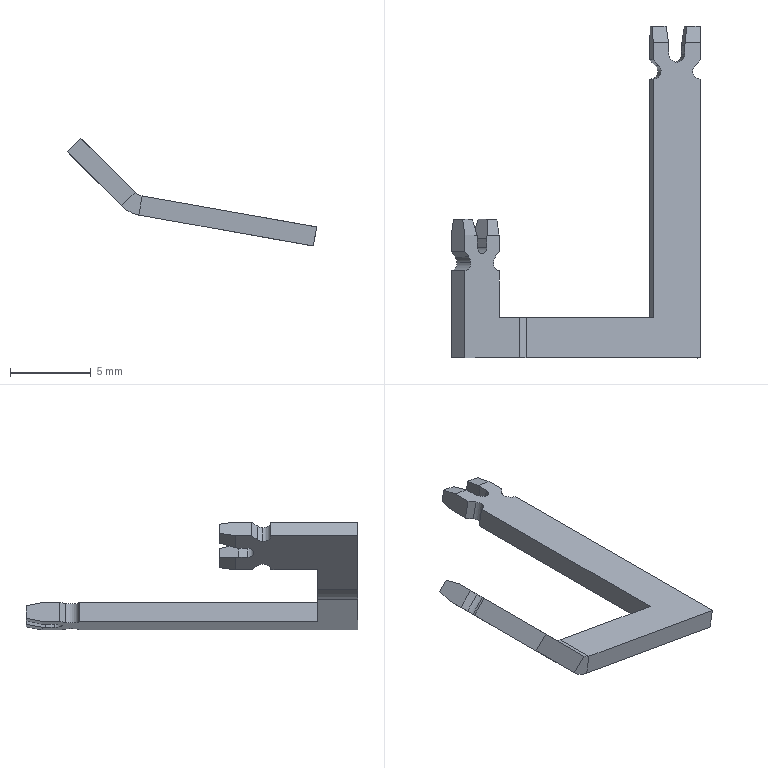Part | SolidWorks | features BaseBody 1 | 1 solid | 52 faces | box 15.479 x 20.6 x 6.702 mm | volume 129.141 mm3 | plane 42 | cylinder 10 | commonest cylinder face diameters 1 x7 0.8 x1 1.64 x1 4.04 x1